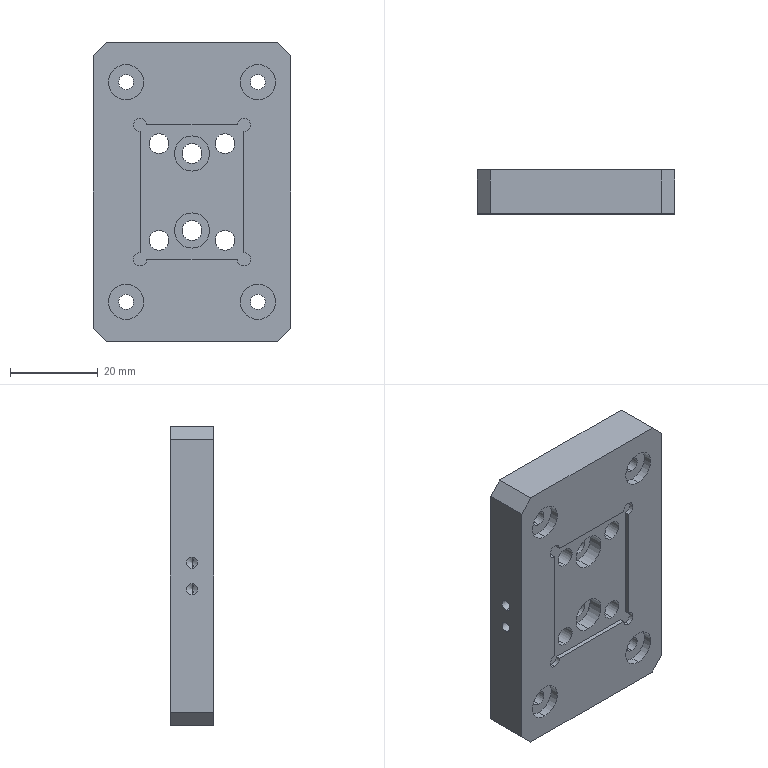Part | STEP file | PN_0038 | 1 solid | 113 faces | box 45 x 10 x 68 mm | volume 26101 mm3 | cylinder 73 | plane 30 | cone 10 | commonest cylinder face diameters 8 x20 4.5 x12 1.5 x8 3.4 x8 6.5 x8 3 x6